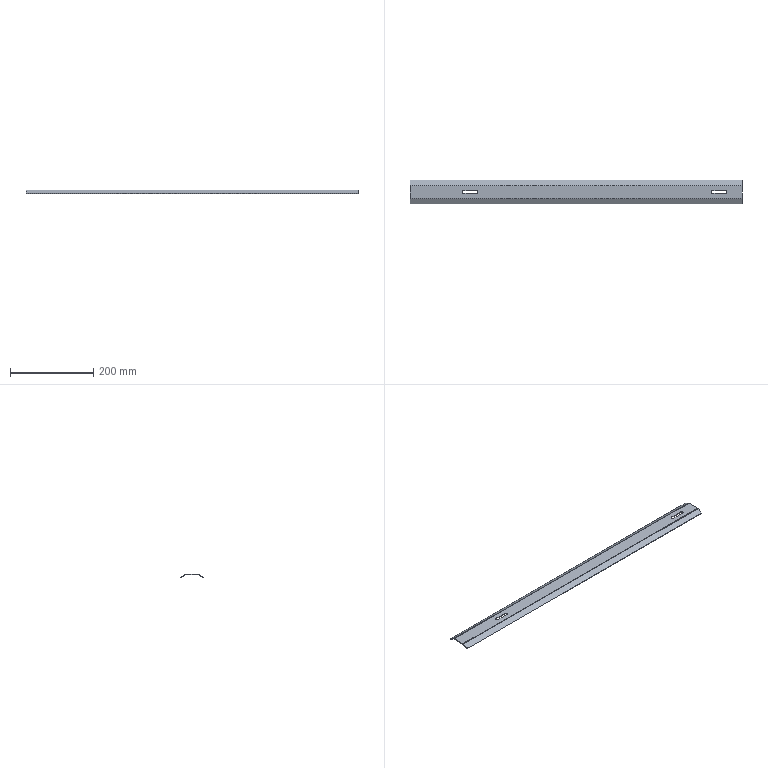Part | STEP file | PN_0012_chain cover plate | 1 solid | 24 faces | box 800 x 57.053 x 9.232 mm | volume 94938 mm3 | plane 14 | cylinder 10 | commonest cylinder face diameters 7 x6 1.473 x2 5.473 x2